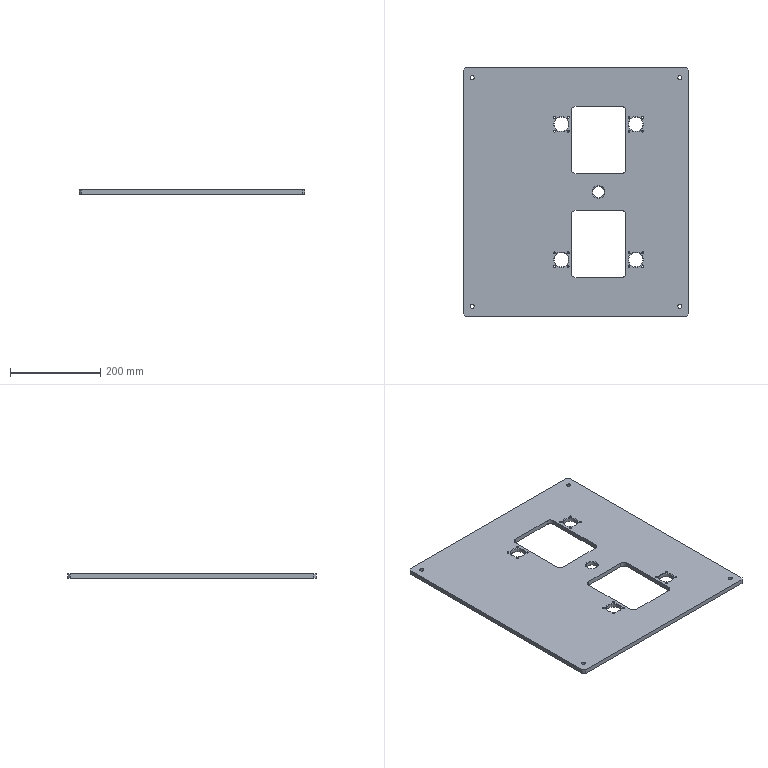Part | 1 solid | 61 faces | box 500 x 550 x 10 mm | volume 2348482 mm3 | cylinder 33 | plane 18 | cone 10 | commonest cylinder face diameters 4.2 x16 20 x8 9 x4 32 x4 26 x1